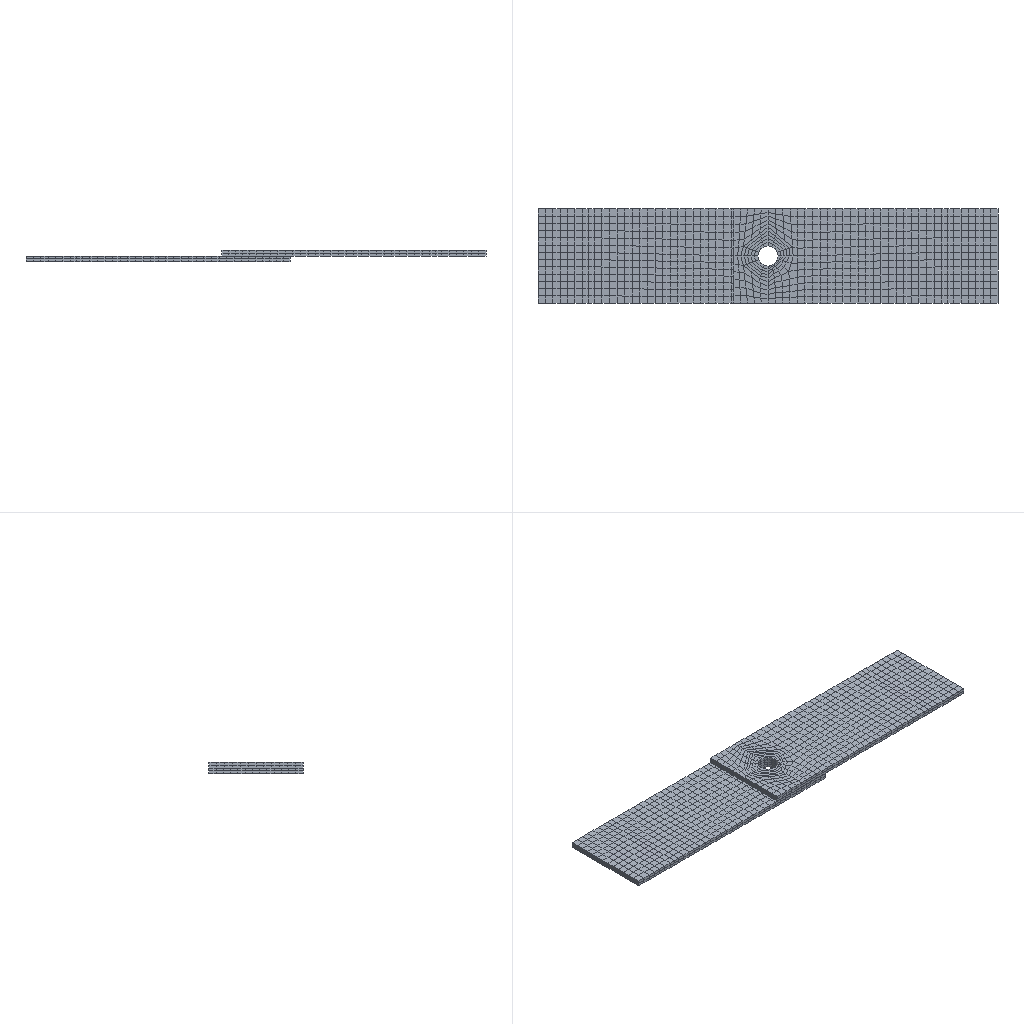Simulation study | abaqus
Set-up summary:
category,name,step,type,value,unit,region
solver,abaqus
solver,version,,,Abaqus/Explicit 2020
units,not stated in the deck,,not stated
analysis,deck,,transient,transient
load_step,Step-1,Step-1,transient
load_step,requested,,,1
mesh,nodes,,,4022
mesh,elements,,,2614
element_type,R3D3,,rigid,6
element_type,R3D4,,rigid,476
element_type,C3D8R,,solid,2132
load,load commands in deck,,count,1
bc,support commands in deck,,count,10
material,MATERIAL-1,,in results
check,setup vs results,,match,"per instance, exact: element labels, types and connectivity; labels of the nodes the elements use; coordinates not compared"
Abaqus input file, long lists of numbers shortened:
*Heading
** Job name: Job-1 Model name: Model-1
** Generated by: Abaqus/CAE 2020
*Preprint, echo=NO, model=NO, history=NO, contact=NO
**
** PARTS
**
*Part, name=ban
*Node
      1,  -15.096,         -25.,           0.
      2,  -15.096,         -25.,          1.5
** (1768 more lines like these left out)
*Element, type=C3D8R
 1,   70,  403, 1360,  379,    1,   39,  377,   42
 2,  403,   83,  391, 1360,   39,    2,   40,  377
** (1064 more lines like these left out)
*Nset, nset=Set-4, generate
    1,  1770,     1
*Elset, elset=Set-4, generate
    1,  1066,     1
** Section: Section-1
*Solid Section, elset=Set-4, material=Material-1
,
*End Part
**
*Part, name=ding
*Node
      1,   2.7,         -2.5,           0.
      2,           4.,           0.,           0.
** (479 more lines like these left out)
*Element, type=R3D4
 1,   1,  27, 128,  28
 2,  27,  26, 129, 128
** (474 more lines like these left out)
*Element, type=R3D3
369, 405, 424, 404
424, 448, 459, 436
** (4 more lines like these left out)
*Node
    482,           0.,           0., 2.44929371e-16
*Nset, nset=ding-RefPt_, internal
482,
*Elset, elset=ding, generate
   1,  482,    1
*End Part
**
**
** ASSEMBLY
**
*Assembly, name=Assembly
**
*Instance, name=ban-1, part=ban
*End Instance
**
*Instance, name=ding-1, part=ding
       30.97,        -12.5,          5.5
       30.97,        -12.5,          5.5, 31.97,        -12.5,          5.5, 90.
*End Instance
**
*Instance, name=ban-2, part=ban
       61.94,           0.,           3.
       61.94,           0.,           3.,        61.94,           1.,           3.,         180.
*End Instance
**
*Nset, nset=Set-1, instance=ding-1
 482,
*Nset, nset=Set-2, instance=ban-1
    1,    2,    3,    4,    5,    6,    7,    8,    9,   10,   13,   14,   15,   16,   17,   18
   20,   22,   27,   28,   33,   34,   35,   38,   39,   40,   41,   42,   43,   44,   45,   46
** (12 more lines like these left out)
*Nset, nset=Set-2, instance=ban-2
    1,    2,    3,    4,    5,    6,    7,    8,    9,   10,   13,   14,   15,   16,   17,   18
   20,   22,   27,   28,   33,   34,   35,   38,   39,   40,   41,   42,   43,   44,   45,   46
** (12 more lines like these left out)
*Elset, elset=Set-2, instance=ban-1
    1,    2,    3,    4,   49,   50,   51,   52,   53,   54,   77,   78,   79,   80,  103,  104
  105,  106,  129,  130,  131,  132,  155,  156,  157,  158,  181,  182,  183,  184,  207,  208
** (7 more lines like these left out)
*Elset, elset=Set-2, instance=ban-2
    1,    2,    3,    4,   49,   50,   51,   52,   53,   54,   77,   78,   79,   80,  103,  104
  105,  106,  129,  130,  131,  132,  155,  156,  157,  158,  181,  182,  183,  184,  207,  208
** (7 more lines like these left out)
*Nset, nset=Set-3, instance=ban-1
  15,  16,  17,  18, 192, 193, 194, 195, 196, 197, 198, 199, 200, 201, 202, 203
 204, 205, 206, 207, 208, 209, 210, 211, 212, 213, 214, 215, 216, 217, 906, 907
** (1 more lines like these left out)
*Elset, elset=Set-3, instance=ban-1, generate
 547,  572,    1
*Nset, nset=Set-4, instance=ban-2
  15,  16,  17,  18, 192, 193, 194, 195, 196, 197, 198, 199, 200, 201, 202, 203
 204, 205, 206, 207, 208, 209, 210, 211, 212, 213, 214, 215, 216, 217, 906, 907
** (1 more lines like these left out)
*Elset, elset=Set-4, instance=ban-2, generate
 547,  572,    1
*Nset, nset=Set-5, instance=ban-1
    3,    4,    6,    7,   15,   16,   17,   18,   41,   45,   47,   48,   49,   50,   51,   52
   53,   54,   55,   56,   57,   58,   71,   72,   73,   74,   75,   76,   77,   78,   79,   80
** (17 more lines like these left out)
*Elset, elset=Set-5, instance=ban-1, generate
 547,  702,    1
*Nset, nset=Set-6, instance=ban-1
    1,    2,    3,    4,    5,    6,    7,    8,    9,   10,   13,   14,   15,   16,   17,   18
   20,   22,   27,   28,   33,   34,   35,   38,   39,   40,   41,   42,   43,   44,   45,   46
** (12 more lines like these left out)
*Nset, nset=Set-6, instance=ban-2
    1,    2,    3,    4,    5,    6,    7,    8,    9,   10,   13,   14,   20,   22,   27,   28
   33,   34,   35,   38,   39,   40,   41,   42,   43,   44,   45,   46,   95,  109,  120,  121
** (10 more lines like these left out)
*Elset, elset=Set-6, instance=ban-1
    1,    2,    3,    4,   49,   50,   51,   52,   53,   54,   77,   78,   79,   80,  103,  104
  105,  106,  129,  130,  131,  132,  155,  156,  157,  158,  181,  182,  183,  184,  207,  208
** (7 more lines like these left out)
*Elset, elset=Set-6, instance=ban-2
    1,    2,    3,    4,   49,   50,   51,   52,   53,   54,   77,   78,   79,   80,  103,  104
  105,  106,  129,  130,  131,  132,  155,  156,  157,  158,  181,  182,  183,  184,  207,  208
** (6 more lines like these left out)
*Nset, nset=Set-7, instance=ban-1
   10,   11,   13,   22,   23,   24,   28,   29,   30,   35,   36,   37,   38,   96,   97,   98
   99,  100,  101,  115,  116,  117,  118,  119,  261,  262,  263,  264,  265,  266,  267,  268
** (12 more lines like these left out)
*Elset, elset=Set-7, instance=ban-1
  744,  745,  746,  747,  748,  749,  750,  751,  752,  753,  754,  755,  756,  757,  758,  759
  760,  761,  762,  763,  764,  765,  766,  767,  768,  769,  770,  771,  772,  773,  774,  775
** (10 more lines like these left out)
*Nset, nset=Set-8, instance=ban-2
    3,    4,    6,    7,   15,   16,   17,   18,   41,   45,   47,   48,   49,   50,   51,   52
   53,   54,   55,   56,   57,   58,   71,   72,   73,   74,   75,   76,   77,   78,   79,   80
** (17 more lines like these left out)
*Elset, elset=Set-8, instance=ban-2, generate
 547,  702,    1
*Nset, nset=Set-9, instance=ban-1
    1,    2,    3,    4,    5,    6,    7,    8,    9,   10,   13,   14,   15,   16,   17,   18
   20,   22,   27,   28,   33,   34,   35,   38,   39,   40,   41,   42,   43,   44,   45,   46
** (12 more lines like these left out)
*Nset, nset=Set-9, instance=ban-2
    1,    2,    5,    8,    9,   10,   13,   14,   20,   22,   27,   28,   33,   34,   35,   38
   39,   43,   95,  109,  120,  121,  122,  123,  124,  125,  126,  127,  128,  129,  130,  131
** (9 more lines like these left out)
*Elset, elset=Set-9, instance=ban-1
    1,    2,    3,    4,   49,   50,   51,   52,   53,   54,   77,   78,   79,   80,  103,  104
  105,  106,  129,  130,  131,  132,  155,  156,  157,  158,  181,  182,  183,  184,  207,  208
** (7 more lines like these left out)
*Elset, elset=Set-9, instance=ban-2
   53,   54,   77,   78,   79,   80,  103,  104,  105,  106,  129,  130,  131,  132,  155,  156
  157,  158,  181,  182,  183,  184,  207,  208,  209,  210,  233,  234,  235,  236,  259,  260
** (5 more lines like these left out)
*Elset, elset=_m_Surf-1_SPOS, internal, instance=ding-1
   1,   2,   3,   4,   5,   6,   7,   8,   9,  10,  11,  12,  13,  14,  15,  16
  17,  18,  19,  20,  21,  22,  23,  24,  25,  26,  27,  28,  29,  30,  31,  32
** (25 more lines like these left out)
*Surface, type=ELEMENT, name=m_Surf-1
_m_Surf-1_SPOS, SPOS
*Elset, elset=_m_Surf-4_S1, internal, instance=ban-1
  703,  704,  705,  706,  707,  708,  709,  710,  711,  712,  713,  714,  715,  716,  717,  718
  719,  720,  721,  722,  723,  724,  725,  726,  727,  728,  729,  730,  731,  732,  733,  734
** (10 more lines like these left out)
*Elset, elset=_m_Surf-4_S4, internal, instance=ban-1
   2,   4,   6,   8,  10,  12,  14,  16,  18,  20,  22,  24,  26,  28,  30,  32
  34,  36,  38,  40,  42,  44,  46,  48,  50,  52, 548, 550, 552, 554, 556, 558
** (5 more lines like these left out)
*Elset, elset=_m_Surf-4_S6, internal, instance=ban-1, generate
  53,  545,    2
*Surface, type=ELEMENT, name=m_Surf-4
_m_Surf-4_S1, S1
_m_Surf-4_S4, S4
_m_Surf-4_S6, S6
*Elset, elset=_s_Surf-1_S4, internal, instance=ban-1
  743,  784,  804,  809,  814,  851,  856,  861,  925,  972,  992,  997, 1002, 1039, 1044, 1049
*Elset, elset=_s_Surf-1_S5, internal, instance=ban-1
  703,  704,  705,  744,  745,  746,  815,  862, 1003, 1004, 1050, 1051
*Elset, elset=_s_Surf-1_S6, internal, instance=ban-1
 879, 884, 889, 926, 931, 936
*Surface, type=ELEMENT, name=s_Surf-1
_s_Surf-1_S4, S4
_s_Surf-1_S5, S5
_s_Surf-1_S6, S6
*Elset, elset=_s_Surf-3_S4, internal, instance=ban-2
  743,  784,  804,  809,  814,  851,  856,  861,  925,  972,  992,  997, 1002, 1039, 1044, 1049
*Elset, elset=_s_Surf-3_S5, internal, instance=ban-2
  703,  704,  705,  744,  745,  746,  815,  862, 1003, 1004, 1050, 1051
*Elset, elset=_s_Surf-3_S6, internal, instance=ban-2
 879, 884, 889, 926, 931, 936
*Surface, type=ELEMENT, name=s_Surf-3
_s_Surf-3_S4, S4
_s_Surf-3_S5, S5
_s_Surf-3_S6, S6
*Elset, elset=_s_Surf-4_S2, internal, instance=ban-2
  744,  745,  746,  747,  748,  749,  750,  751,  752,  753,  754,  755,  756,  757,  758,  759
  760,  761,  762,  763,  764,  765,  766,  767,  768,  769,  770,  771,  772,  773,  774,  775
** (10 more lines like these left out)
*Elset, elset=_s_Surf-4_S6, internal, instance=ban-2
   1,   3,   5,   7,   9,  11,  13,  15,  17,  19,  21,  23,  25,  27,  29,  31
  33,  35,  37,  39,  41,  43,  45,  47,  49,  51, 547, 549, 551, 553, 555, 557
** (5 more lines like these left out)
*Elset, elset=_s_Surf-4_S4, internal, instance=ban-2, generate
  54,  546,    2
*Surface, type=ELEMENT, name=s_Surf-4
_s_Surf-4_S2, S2
_s_Surf-4_S6, S6
_s_Surf-4_S4, S4
*Rigid Body, ref node=ding-1.ding-RefPt_, elset=ding-1.ding
*End Assembly
*Amplitude, name=Amp-1
             0.,              0.,           0.001,              1.
**
** MATERIALS
**
*Material, name=Material-1
*Damage Initiation, criterion=SHEAR
 0.1,0.,0.
*Damage Evolution, type=DISPLACEMENT
 0.0001,
*Density
 7.8e-09,
*Elastic
210000., 0.3
*Plastic
550.,0.
**
** INTERACTION PROPERTIES
**
*Surface Interaction, name=IntProp-1
*Friction
 0.3,
*Surface Behavior, pressure-overclosure=HARD
**
** BOUNDARY CONDITIONS
**
** Name: BC-1 Type: 对称/反对称/完全固定
*Boundary
Set-1, ENCASTRE
** Name: BC-2 Type: 位移/转角
*Boundary
Set-9, 2, 2
**
** INTERACTIONS
**
** Interaction: Int-4
*Contact, op=NEW
*Contact Inclusions, ALL EXTERIOR
*Contact Property Assignment
 ,  , IntProp-1
** ----------------------------------------------------------------
**
** STEP: Step-1
**
*Step, name=Step-1, nlgeom=YES
*Dynamic, Explicit
, 0.001
*Bulk Viscosity
0.06, 1.2
**
** BOUNDARY CONDITIONS
**
** Name: BC-3 Type: 对称/反对称/完全固定
*Boundary
Set-5, ENCASTRE
** Name: BC-4 Type: 位移/转角
*Boundary, amplitude=Amp-1
Set-8, 1, 1, 15.
Set-8, 2, 2
Set-8, 3, 3
Set-8, 4, 4
Set-8, 5, 5
Set-8, 6, 6
** Name: BC-5 Type: 位移/转角
*Boundary
Set-7, 3, 3
**
** OUTPUT REQUESTS
**
*Restart, write, number interval=1, time marks=NO
**
** FIELD OUTPUT: F-Output-1
**
*Output, field, number interval=50
*Node Output
A, RF, RT, U, V
*Element Output, directions=YES
E, EVF, LE, MISES, PE, PEEQ, PEEQVAVG, PEVAVG, S, STATUS, SVAVG
*Contact Output
CSTRESS,
**
** HISTORY OUTPUT: H-Output-1
**
*Output, history, variable=PRESELECT
*End Step
Results summary:
result,step,Step-1,completed,increments=17757 time=0.001/0.001
result,analysis,,,transient
result,last_loadstep,,,1
result,primary field,,,U
result,reaction total,,FX,-8008.661,model units
result,reaction total,,FY,4042.357,model units
result,reaction total,,FZ,18.661,model units